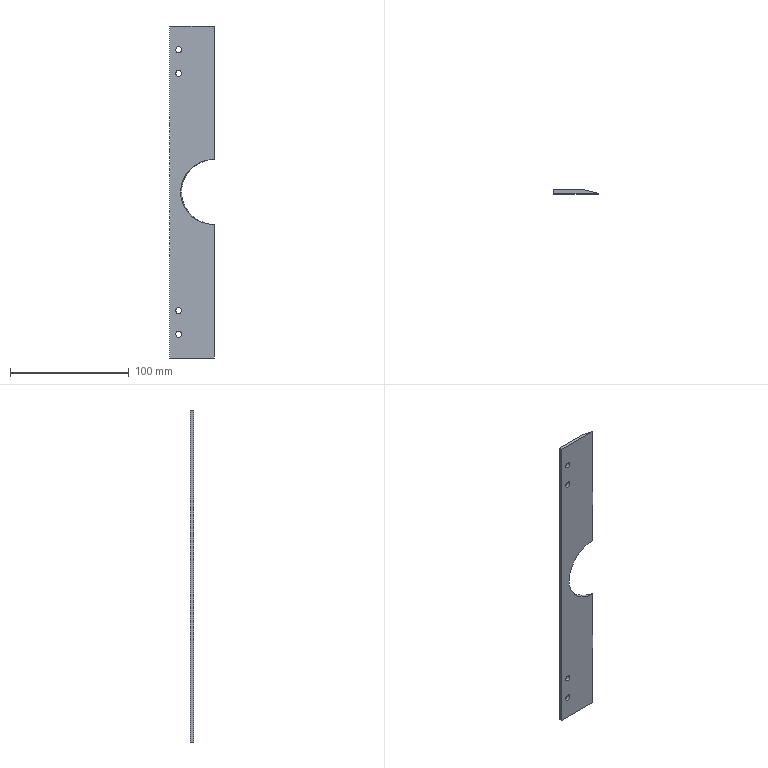Part | SolidWorks | features Cut 1, Extrusion 1, ICE 1 | 1 solid | 17 faces | box 37.5 x 3 x 280 mm | volume 23848 mm3 | cylinder 10 | plane 7 | commonest cylinder face diameters 5 x8 55 x2
STEP:
#1=CARTESIAN_POINT('',(9.03,-3.,140.));
#2=VERTEX_POINT('',#1);
#3=CARTESIAN_POINT('',(37.5,-3.,167.5));
#4=VERTEX_POINT('',#3);
#5=CARTESIAN_POINT('',(9.03,-3.,140.));
#6=CARTESIAN_POINT('',(9.03,-3.,156.109));
#7=CARTESIAN_POINT('',(20.823,-3.,167.5));
#8=CARTESIAN_POINT('',(37.5,-3.,167.5));
#9=(BOUNDED_CURVE()B_SPLINE_CURVE(3,(#5,#6,#7,#8),.UNSPECIFIED.,.F.,.F.)B_SPLINE_CURVE_WITH_KNOTS((4,4),(3.142,4.712),.UNSPECIFIED.)CURVE()GEOMETRIC_REPRESENTATION_ITEM()RATIONAL_B_SPLINE_CURVE((1.,0.8047,0.8047,1.))REPRESENTATION_ITEM(''));
#10=EDGE_CURVE('',#2,#4,#9,.T.);
#11=ORIENTED_EDGE('',*,*,#10,.F.);
#12=CARTESIAN_POINT('',(9.834,0.,140.));
#13=VERTEX_POINT('',#12);
#14=CARTESIAN_POINT('',(8.425,-5.257,140.));
#15=DIRECTION('',(0.2588,0.9659,0.));
#16=VECTOR('',#15,1000.);
#17=LINE('',#14,#16);
#18=EDGE_CURVE('',#2,#13,#17,.T.);
#19=ORIENTED_EDGE('',*,*,#18,.T.);
#20=CARTESIAN_POINT('',(26.304,0.,164.938));
#21=VERTEX_POINT('',#20);
#22=CARTESIAN_POINT('',(26.304,0.,164.938));
#23=CARTESIAN_POINT('',(15.965,0.,160.296));
#24=CARTESIAN_POINT('',(9.834,0.,151.012));
#25=CARTESIAN_POINT('',(9.834,0.,140.));
#26=(BOUNDED_CURVE()B_SPLINE_CURVE(3,(#22,#23,#24,#25),.UNSPECIFIED.,.F.,.F.)B_SPLINE_CURVE_WITH_KNOTS((4,4),(2.006,3.142),.UNSPECIFIED.)CURVE()GEOMETRIC_REPRESENTATION_ITEM()RATIONAL_B_SPLINE_CURVE((1.,0.8954,0.8954,1.))REPRESENTATION_ITEM(''));
#27=EDGE_CURVE('',#21,#13,#26,.T.);
#28=ORIENTED_EDGE('',*,*,#27,.F.);
#29=CARTESIAN_POINT('',(37.5,-3.,140.));
#30=DIRECTION('',(0.2588,0.9659,0.));
#31=DIRECTION('',(-0.9659,0.2588,0.));
#32=AXIS2_PLACEMENT_3D('',#29,#30,#31);
#33=CIRCLE('',#32,27.5);
#34=EDGE_CURVE('',#21,#4,#33,.T.);
#35=ORIENTED_EDGE('',*,*,#34,.T.);
#36=EDGE_LOOP('',(#11,#19,#28,#35));
#37=FACE_OUTER_BOUND('',#36,.T.);
#38=CARTESIAN_POINT('',(34.988,-12.375,140.));
#39=DIRECTION('',(0.2588,0.9659,0.));
#40=DIRECTION('',(-0.9659,0.2588,0.));
#41=AXIS2_PLACEMENT_3D('',#38,#39,#40);
#42=CYLINDRICAL_SURFACE('',#41,27.5);
#43=ADVANCED_FACE('',(#37),#42,.F.);
#44=CARTESIAN_POINT('',(10.,-3.,260.));
#45=VERTEX_POINT('',#44);
#46=CARTESIAN_POINT('',(5.,-3.,260.));
#47=VERTEX_POINT('',#46);
#48=CARTESIAN_POINT('',(7.5,-3.,260.));
#49=DIRECTION('',(0.,1.,0.));
#50=DIRECTION('',(0.,0.,1.));
#51=AXIS2_PLACEMENT_3D('',#48,#49,#50);
#52=CIRCLE('',#51,2.5);
#53=EDGE_CURVE('',#45,#47,#52,.T.);
#54=ORIENTED_EDGE('',*,*,#53,.F.);
#55=CARTESIAN_POINT('',(10.,0.,260.));
#56=VERTEX_POINT('',#55);
#57=CARTESIAN_POINT('',(10.,-280.,260.));
#58=DIRECTION('',(0.,1.,0.));
#59=VECTOR('',#58,1000.);
#60=LINE('',#57,#59);
#61=EDGE_CURVE('',#45,#56,#60,.T.);
#62=ORIENTED_EDGE('',*,*,#61,.T.);
#63=CARTESIAN_POINT('',(5.,0.,260.));
#64=VERTEX_POINT('',#63);
#65=CARTESIAN_POINT('',(7.5,0.,260.));
#66=DIRECTION('',(0.,1.,0.));
#67=DIRECTION('',(-1.,0.,0.));
#68=AXIS2_PLACEMENT_3D('',#65,#66,#67);
#69=CIRCLE('',#68,2.5);
#70=EDGE_CURVE('',#56,#64,#69,.T.);
#71=ORIENTED_EDGE('',*,*,#70,.T.);
#72=CARTESIAN_POINT('',(5.,-280.,260.));
#73=DIRECTION('',(0.,1.,0.));
#74=VECTOR('',#73,1000.);
#75=LINE('',#72,#74);
#76=EDGE_CURVE('',#47,#64,#75,.T.);
#77=ORIENTED_EDGE('',*,*,#76,.F.);
#78=EDGE_LOOP('',(#54,#62,#71,#77));
#79=FACE_OUTER_BOUND('',#78,.T.);
#80=CARTESIAN_POINT('',(7.5,-280.,260.));
#81=DIRECTION('',(0.,1.,0.));
#82=DIRECTION('',(-1.,0.,0.));
#83=AXIS2_PLACEMENT_3D('',#80,#81,#82);
#84=CYLINDRICAL_SURFACE('',#83,2.5);
#85=ADVANCED_FACE('',(#79),#84,.F.);
#86=CARTESIAN_POINT('',(10.,-3.,40.));
#87=VERTEX_POINT('',#86);
#88=CARTESIAN_POINT('',(5.,-3.,40.));
#89=VERTEX_POINT('',#88);
#90=CARTESIAN_POINT('',(7.5,-3.,40.));
#91=DIRECTION('',(0.,1.,0.));
#92=DIRECTION('',(0.,0.,1.));
#93=AXIS2_PLACEMENT_3D('',#90,#91,#92);
#94=CIRCLE('',#93,2.5);
#95=EDGE_CURVE('',#87,#89,#94,.T.);
#96=ORIENTED_EDGE('',*,*,#95,.F.);
#97=CARTESIAN_POINT('',(10.,0.,40.));
#98=VERTEX_POINT('',#97);
#99=CARTESIAN_POINT('',(10.,-280.,40.));
#100=DIRECTION('',(0.,1.,0.));
#101=VECTOR('',#100,1000.);
#102=LINE('',#99,#101);
#103=EDGE_CURVE('',#87,#98,#102,.T.);
#104=ORIENTED_EDGE('',*,*,#103,.T.);
#105=CARTESIAN_POINT('',(5.,0.,40.));
#106=VERTEX_POINT('',#105);
#107=CARTESIAN_POINT('',(7.5,0.,40.));
#108=DIRECTION('',(0.,1.,0.));
#109=DIRECTION('',(-1.,0.,0.));
#110=AXIS2_PLACEMENT_3D('',#107,#108,#109);
#111=CIRCLE('',#110,2.5);
#112=EDGE_CURVE('',#98,#106,#111,.T.);
#113=ORIENTED_EDGE('',*,*,#112,.T.);
#114=CARTESIAN_POINT('',(5.,-280.,40.));
#115=DIRECTION('',(0.,1.,0.));
#116=VECTOR('',#115,1000.);
#117=LINE('',#114,#116);
#118=EDGE_CURVE('',#89,#106,#117,.T.);
#119=ORIENTED_EDGE('',*,*,#118,.F.);
#120=EDGE_LOOP('',(#96,#104,#113,#119));
#121=FACE_OUTER_BOUND('',#120,.T.);
#122=CARTESIAN_POINT('',(7.5,-280.,40.));
#123=DIRECTION('',(0.,1.,0.));
#124=DIRECTION('',(-1.,0.,0.));
#125=AXIS2_PLACEMENT_3D('',#122,#123,#124);
#126=CYLINDRICAL_SURFACE('',#125,2.5);
#127=ADVANCED_FACE('',(#121),#126,.F.);
#128=CARTESIAN_POINT('',(10.,-3.,20.));
#129=VERTEX_POINT('',#128);
#130=CARTESIAN_POINT('',(5.,-3.,20.));
#131=VERTEX_POINT('',#130);
#132=CARTESIAN_POINT('',(7.5,-3.,20.));
#133=DIRECTION('',(0.,1.,0.));
#134=DIRECTION('',(0.,0.,1.));
#135=AXIS2_PLACEMENT_3D('',#132,#133,#134);
#136=CIRCLE('',#135,2.5);
#137=EDGE_CURVE('',#129,#131,#136,.T.);
#138=ORIENTED_EDGE('',*,*,#137,.F.);
#139=CARTESIAN_POINT('',(10.,0.,20.));
#140=VERTEX_POINT('',#139);
#141=CARTESIAN_POINT('',(10.,-280.,20.));
#142=DIRECTION('',(0.,1.,0.));
#143=VECTOR('',#142,1000.);
#144=LINE('',#141,#143);
#145=EDGE_CURVE('',#129,#140,#144,.T.);
#146=ORIENTED_EDGE('',*,*,#145,.T.);
#147=CARTESIAN_POINT('',(5.,0.,20.));
#148=VERTEX_POINT('',#147);
#149=CARTESIAN_POINT('',(7.5,0.,20.));
#150=DIRECTION('',(0.,1.,0.));
#151=DIRECTION('',(-1.,0.,0.));
#152=AXIS2_PLACEMENT_3D('',#149,#150,#151);
#153=CIRCLE('',#152,2.5);
#154=EDGE_CURVE('',#140,#148,#153,.T.);
#155=ORIENTED_EDGE('',*,*,#154,.T.);
#156=CARTESIAN_POINT('',(5.,-280.,20.));
#157=DIRECTION('',(0.,1.,0.));
#158=VECTOR('',#157,1000.);
#159=LINE('',#156,#158);
#160=EDGE_CURVE('',#131,#148,#159,.T.);
#161=ORIENTED_EDGE('',*,*,#160,.F.);
#162=EDGE_LOOP('',(#138,#146,#155,#161));
#163=FACE_OUTER_BOUND('',#162,.T.);
#164=CARTESIAN_POINT('',(7.5,-280.,20.));
#165=DIRECTION('',(0.,1.,0.));
#166=DIRECTION('',(-1.,0.,0.));
#167=AXIS2_PLACEMENT_3D('',#164,#165,#166);
#168=CYLINDRICAL_SURFACE('',#167,2.5);
#169=ADVANCED_FACE('',(#163),#168,.F.);
#170=CARTESIAN_POINT('',(10.,-3.,240.));
#171=VERTEX_POINT('',#170);
#172=CARTESIAN_POINT('',(5.,-3.,240.));
#173=VERTEX_POINT('',#172);
#174=CARTESIAN_POINT('',(7.5,-3.,240.));
#175=DIRECTION('',(0.,1.,0.));
#176=DIRECTION('',(0.,0.,1.));
#177=AXIS2_PLACEMENT_3D('',#174,#175,#176);
#178=CIRCLE('',#177,2.5);
#179=EDGE_CURVE('',#171,#173,#178,.T.);
#180=ORIENTED_EDGE('',*,*,#179,.F.);
#181=CARTESIAN_POINT('',(10.,0.,240.));
#182=VERTEX_POINT('',#181);
#183=CARTESIAN_POINT('',(10.,-280.,240.));
#184=DIRECTION('',(0.,1.,0.));
#185=VECTOR('',#184,1000.);
#186=LINE('',#183,#185);
#187=EDGE_CURVE('',#171,#182,#186,.T.);
#188=ORIENTED_EDGE('',*,*,#187,.T.);
#189=CARTESIAN_POINT('',(5.,0.,240.));
#190=VERTEX_POINT('',#189);
#191=CARTESIAN_POINT('',(7.5,0.,240.));
#192=DIRECTION('',(0.,1.,0.));
#193=DIRECTION('',(-1.,0.,0.));
#194=AXIS2_PLACEMENT_3D('',#191,#192,#193);
#195=CIRCLE('',#194,2.5);
#196=EDGE_CURVE('',#182,#190,#195,.T.);
#197=ORIENTED_EDGE('',*,*,#196,.T.);
#198=CARTESIAN_POINT('',(5.,-280.,240.));
#199=DIRECTION('',(0.,1.,0.));
#200=VECTOR('',#199,1000.);
#201=LINE('',#198,#200);
#202=EDGE_CURVE('',#173,#190,#201,.T.);
#203=ORIENTED_EDGE('',*,*,#202,.F.);
#204=EDGE_LOOP('',(#180,#188,#197,#203));
#205=FACE_OUTER_BOUND('',#204,.T.);
#206=CARTESIAN_POINT('',(7.5,-280.,240.));
#207=DIRECTION('',(0.,1.,0.));
#208=DIRECTION('',(-1.,0.,0.));
#209=AXIS2_PLACEMENT_3D('',#206,#207,#208);
#210=CYLINDRICAL_SURFACE('',#209,2.5);
#211=ADVANCED_FACE('',(#205),#210,.F.);
#212=CARTESIAN_POINT('',(37.5,-3.,280.));
#213=VERTEX_POINT('',#212);
#214=CARTESIAN_POINT('',(37.5,-3.,280.));
#215=DIRECTION('',(0.,0.,-1.));
#216=VECTOR('',#215,1000.);
#217=LINE('',#214,#216);
#218=EDGE_CURVE('',#213,#4,#217,.T.);
#219=ORIENTED_EDGE('',*,*,#218,.T.);
#220=ORIENTED_EDGE('',*,*,#34,.F.);
#221=CARTESIAN_POINT('',(26.304,0.,280.));
#222=VERTEX_POINT('',#221);
#223=CARTESIAN_POINT('',(26.304,0.,280.));
#224=DIRECTION('',(0.,0.,-1.));
#225=VECTOR('',#224,1000.);
#226=LINE('',#223,#225);
#227=EDGE_CURVE('',#222,#21,#226,.T.);
#228=ORIENTED_EDGE('',*,*,#227,.F.);
#229=CARTESIAN_POINT('',(37.5,-3.,280.));
#230=DIRECTION('',(-0.9659,0.2588,0.));
#231=VECTOR('',#230,1000.);
#232=LINE('',#229,#231);
#233=EDGE_CURVE('',#213,#222,#232,.T.);
#234=ORIENTED_EDGE('',*,*,#233,.F.);
#235=EDGE_LOOP('',(#219,#220,#228,#234));
#236=FACE_OUTER_BOUND('',#235,.T.);
#237=CARTESIAN_POINT('',(37.5,-3.,280.));
#238=DIRECTION('',(-0.2588,-0.9659,0.));
#239=DIRECTION('',(0.9659,-0.2588,0.));
#240=AXIS2_PLACEMENT_3D('',#237,#238,#239);
#241=PLANE('',#240);
#242=ADVANCED_FACE('',(#236),#241,.F.);
#243=CARTESIAN_POINT('',(7.5,0.,260.));
#244=DIRECTION('',(0.,1.,0.));
#245=DIRECTION('',(-1.,0.,0.));
#246=AXIS2_PLACEMENT_3D('',#243,#244,#245);
#247=CIRCLE('',#246,2.5);
#248=EDGE_CURVE('',#64,#56,#247,.T.);
#249=ORIENTED_EDGE('',*,*,#248,.F.);
#250=ORIENTED_EDGE('',*,*,#70,.F.);
#251=EDGE_LOOP('',(#249,#250));
#252=FACE_BOUND('',#251,.T.);
#253=CARTESIAN_POINT('',(7.5,0.,40.));
#254=DIRECTION('',(0.,1.,0.));
#255=DIRECTION('',(-1.,0.,0.));
#256=AXIS2_PLACEMENT_3D('',#253,#254,#255);
#257=CIRCLE('',#256,2.5);
#258=EDGE_CURVE('',#106,#98,#257,.T.);
#259=ORIENTED_EDGE('',*,*,#258,.F.);
#260=ORIENTED_EDGE('',*,*,#112,.F.);
#261=EDGE_LOOP('',(#259,#260));
#262=FACE_BOUND('',#261,.T.);
#263=CARTESIAN_POINT('',(7.5,0.,20.));
#264=DIRECTION('',(0.,1.,0.));
#265=DIRECTION('',(-1.,0.,0.));
#266=AXIS2_PLACEMENT_3D('',#263,#264,#265);
#267=CIRCLE('',#266,2.5);
#268=EDGE_CURVE('',#148,#140,#267,.T.);
#269=ORIENTED_EDGE('',*,*,#268,.F.);
#270=ORIENTED_EDGE('',*,*,#154,.F.);
#271=EDGE_LOOP('',(#269,#270));
#272=FACE_BOUND('',#271,.T.);
#273=CARTESIAN_POINT('',(7.5,0.,240.));
#274=DIRECTION('',(0.,1.,0.));
#275=DIRECTION('',(-1.,0.,0.));
#276=AXIS2_PLACEMENT_3D('',#273,#274,#275);
#277=CIRCLE('',#276,2.5);
#278=EDGE_CURVE('',#190,#182,#277,.T.);
#279=ORIENTED_EDGE('',*,*,#278,.F.);
#280=ORIENTED_EDGE('',*,*,#196,.F.);
#281=EDGE_LOOP('',(#279,#280));
#282=FACE_BOUND('',#281,.T.);
#283=ORIENTED_EDGE('',*,*,#227,.T.);
#284=ORIENTED_EDGE('',*,*,#27,.T.);
#285=CARTESIAN_POINT('',(26.304,0.,115.062));
#286=VERTEX_POINT('',#285);
#287=CARTESIAN_POINT('',(9.834,0.,140.));
#288=CARTESIAN_POINT('',(9.834,0.,128.988));
#289=CARTESIAN_POINT('',(15.965,0.,119.704));
#290=CARTESIAN_POINT('',(26.304,0.,115.062));
#291=(BOUNDED_CURVE()B_SPLINE_CURVE(3,(#287,#288,#289,#290),.UNSPECIFIED.,.F.,.F.)B_SPLINE_CURVE_WITH_KNOTS((4,4),(3.142,4.277),.UNSPECIFIED.)CURVE()GEOMETRIC_REPRESENTATION_ITEM()RATIONAL_B_SPLINE_CURVE((1.,0.8954,0.8954,1.))REPRESENTATION_ITEM(''));
#292=EDGE_CURVE('',#13,#286,#291,.T.);
#293=ORIENTED_EDGE('',*,*,#292,.T.);
#294=CARTESIAN_POINT('',(26.304,0.,0.));
#295=VERTEX_POINT('',#294);
#296=CARTESIAN_POINT('',(26.304,0.,280.));
#297=DIRECTION('',(0.,0.,-1.));
#298=VECTOR('',#297,1000.);
#299=LINE('',#296,#298);
#300=EDGE_CURVE('',#286,#295,#299,.T.);
#301=ORIENTED_EDGE('',*,*,#300,.T.);
#302=CARTESIAN_POINT('',(0.,0.,0.));
#303=VERTEX_POINT('',#302);
#304=CARTESIAN_POINT('',(26.304,0.,0.));
#305=DIRECTION('',(-1.,0.,0.));
#306=VECTOR('',#305,1000.);
#307=LINE('',#304,#306);
#308=EDGE_CURVE('',#295,#303,#307,.T.);
#309=ORIENTED_EDGE('',*,*,#308,.T.);
#310=CARTESIAN_POINT('',(0.,0.,280.));
#311=VERTEX_POINT('',#310);
#312=CARTESIAN_POINT('',(0.,0.,280.));
#313=DIRECTION('',(0.,0.,-1.));
#314=VECTOR('',#313,1000.);
#315=LINE('',#312,#314);
#316=EDGE_CURVE('',#311,#303,#315,.T.);
#317=ORIENTED_EDGE('',*,*,#316,.F.);
#318=CARTESIAN_POINT('',(26.304,0.,280.));
#319=DIRECTION('',(-1.,0.,0.));
#320=VECTOR('',#319,1000.);
#321=LINE('',#318,#320);
#322=EDGE_CURVE('',#222,#311,#321,.T.);
#323=ORIENTED_EDGE('',*,*,#322,.F.);
#324=EDGE_LOOP('',(#283,#284,#293,#301,#309,#317,#323));
#325=FACE_OUTER_BOUND('',#324,.T.);
#326=CARTESIAN_POINT('',(26.304,0.,280.));
#327=DIRECTION('',(0.,-1.,0.));
#328=DIRECTION('',(1.,0.,0.));
#329=AXIS2_PLACEMENT_3D('',#326,#327,#328);
#330=PLANE('',#329);
#331=ADVANCED_FACE('',(#252,#262,#272,#282,#325),#330,.F.);
#332=CARTESIAN_POINT('',(0.,-3.,0.));
#333=VERTEX_POINT('',#332);
#334=CARTESIAN_POINT('',(0.,0.,0.));
#335=DIRECTION('',(0.,-1.,0.));
#336=VECTOR('',#335,1000.);
#337=LINE('',#334,#336);
#338=EDGE_CURVE('',#303,#333,#337,.T.);
#339=ORIENTED_EDGE('',*,*,#338,.T.);
#340=CARTESIAN_POINT('',(0.,-3.,280.));
#341=VERTEX_POINT('',#340);
#342=CARTESIAN_POINT('',(0.,-3.,280.));
#343=DIRECTION('',(0.,0.,-1.));
#344=VECTOR('',#343,1000.);
#345=LINE('',#342,#344);
#346=EDGE_CURVE('',#341,#333,#345,.T.);
#347=ORIENTED_EDGE('',*,*,#346,.F.);
#348=CARTESIAN_POINT('',(0.,0.,280.));
#349=DIRECTION('',(0.,-1.,0.));
#350=VECTOR('',#349,1000.);
#351=LINE('',#348,#350);
#352=EDGE_CURVE('',#311,#341,#351,.T.);
#353=ORIENTED_EDGE('',*,*,#352,.F.);
#354=ORIENTED_EDGE('',*,*,#316,.T.);
#355=EDGE_LOOP('',(#339,#347,#353,#354));
#356=FACE_OUTER_BOUND('',#355,.T.);
#357=CARTESIAN_POINT('',(0.,0.,280.));
#358=DIRECTION('',(1.,0.,0.));
#359=DIRECTION('',(0.,1.,0.));
#360=AXIS2_PLACEMENT_3D('',#357,#358,#359);
#361=PLANE('',#360);
#362=ADVANCED_FACE('',(#356),#361,.F.);
#363=CARTESIAN_POINT('',(7.5,-3.,260.));
#364=DIRECTION('',(0.,1.,0.));
#365=DIRECTION('',(0.,0.,1.));
#366=AXIS2_PLACEMENT_3D('',#363,#364,#365);
#367=CIRCLE('',#366,2.5);
#368=EDGE_CURVE('',#47,#45,#367,.T.);
#369=ORIENTED_EDGE('',*,*,#368,.T.);
#370=ORIENTED_EDGE('',*,*,#53,.T.);
#371=EDGE_LOOP('',(#369,#370));
#372=FACE_BOUND('',#371,.T.);
#373=CARTESIAN_POINT('',(7.5,-3.,40.));
#374=DIRECTION('',(0.,1.,0.));
#375=DIRECTION('',(0.,0.,1.));
#376=AXIS2_PLACEMENT_3D('',#373,#374,#375);
#377=CIRCLE('',#376,2.5);
#378=EDGE_CURVE('',#89,#87,#377,.T.);
#379=ORIENTED_EDGE('',*,*,#378,.T.);
#380=ORIENTED_EDGE('',*,*,#95,.T.);
#381=EDGE_LOOP('',(#379,#380));
#382=FACE_BOUND('',#381,.T.);
#383=CARTESIAN_POINT('',(7.5,-3.,20.));
#384=DIRECTION('',(0.,1.,0.));
#385=DIRECTION('',(0.,0.,1.));
#386=AXIS2_PLACEMENT_3D('',#383,#384,#385);
#387=CIRCLE('',#386,2.5);
#388=EDGE_CURVE('',#131,#129,#387,.T.);
#389=ORIENTED_EDGE('',*,*,#388,.T.);
#390=ORIENTED_EDGE('',*,*,#137,.T.);
#391=EDGE_LOOP('',(#389,#390));
#392=FACE_BOUND('',#391,.T.);
#393=CARTESIAN_POINT('',(7.5,-3.,240.));
#394=DIRECTION('',(0.,1.,0.));
#395=DIRECTION('',(0.,0.,1.));
#396=AXIS2_PLACEMENT_3D('',#393,#394,#395);
#397=CIRCLE('',#396,2.5);
#398=EDGE_CURVE('',#173,#171,#397,.T.);
#399=ORIENTED_EDGE('',*,*,#398,.T.);
#400=ORIENTED_EDGE('',*,*,#179,.T.);
#401=EDGE_LOOP('',(#399,#400));
#402=FACE_BOUND('',#401,.T.);
#403=CARTESIAN_POINT('',(37.5,-3.,112.5));
#404=VERTEX_POINT('',#403);
#405=CARTESIAN_POINT('',(37.5,-3.,0.));
#406=VERTEX_POINT('',#405);
#407=CARTESIAN_POINT('',(37.5,-3.,280.));
#408=DIRECTION('',(0.,0.,-1.));
#409=VECTOR('',#408,1000.);
#410=LINE('',#407,#409);
#411=EDGE_CURVE('',#404,#406,#410,.T.);
#412=ORIENTED_EDGE('',*,*,#411,.F.);
#413=CARTESIAN_POINT('',(37.5,-3.,112.5));
#414=CARTESIAN_POINT('',(20.823,-3.,112.5));
#415=CARTESIAN_POINT('',(9.03,-3.,123.891));
#416=CARTESIAN_POINT('',(9.03,-3.,140.));
#417=(BOUNDED_CURVE()B_SPLINE_CURVE(3,(#413,#414,#415,#416),.UNSPECIFIED.,.F.,.F.)B_SPLINE_CURVE_WITH_KNOTS((4,4),(1.571,3.142),.UNSPECIFIED.)CURVE()GEOMETRIC_REPRESENTATION_ITEM()RATIONAL_B_SPLINE_CURVE((1.,0.8047,0.8047,1.))REPRESENTATION_ITEM(''));
#418=EDGE_CURVE('',#404,#2,#417,.T.);
#419=ORIENTED_EDGE('',*,*,#418,.T.);
#420=ORIENTED_EDGE('',*,*,#10,.T.);
#421=ORIENTED_EDGE('',*,*,#218,.F.);
#422=CARTESIAN_POINT('',(0.,-3.,280.));
#423=DIRECTION('',(1.,0.,0.));
#424=VECTOR('',#423,1000.);
#425=LINE('',#422,#424);
#426=EDGE_CURVE('',#341,#213,#425,.T.);
#427=ORIENTED_EDGE('',*,*,#426,.F.);
#428=ORIENTED_EDGE('',*,*,#346,.T.);
#429=CARTESIAN_POINT('',(0.,-3.,0.));
#430=DIRECTION('',(1.,0.,0.));
#431=VECTOR('',#430,1000.);
#432=LINE('',#429,#431);
#433=EDGE_CURVE('',#333,#406,#432,.T.);
#434=ORIENTED_EDGE('',*,*,#433,.T.);
#435=EDGE_LOOP('',(#412,#419,#420,#421,#427,#428,#434));
#436=FACE_OUTER_BOUND('',#435,.T.);
#437=CARTESIAN_POINT('',(0.,-3.,280.));
#438=DIRECTION('',(0.,1.,0.));
#439=DIRECTION('',(0.,0.,1.));
#440=AXIS2_PLACEMENT_3D('',#437,#438,#439);
#441=PLANE('',#440);
#442=ADVANCED_FACE('',(#372,#382,#392,#402,#436),#441,.F.);
#443=ORIENTED_EDGE('',*,*,#300,.F.);
#444=CARTESIAN_POINT('',(37.5,-3.,140.));
#445=DIRECTION('',(-0.2588,-0.9659,0.));
#446=DIRECTION('',(0.9659,-0.2588,0.));
#447=AXIS2_PLACEMENT_3D('',#444,#445,#446);
#448=CIRCLE('',#447,27.5);
#449=EDGE_CURVE('',#286,#404,#448,.T.);
#450=ORIENTED_EDGE('',*,*,#449,.T.);
#451=ORIENTED_EDGE('',*,*,#411,.T.);
#452=CARTESIAN_POINT('',(37.5,-3.,0.));
#453=DIRECTION('',(-0.9659,0.2588,0.));
#454=VECTOR('',#453,1000.);
#455=LINE('',#452,#454);
#456=EDGE_CURVE('',#406,#295,#455,.T.);
#457=ORIENTED_EDGE('',*,*,#456,.T.);
#458=EDGE_LOOP('',(#443,#450,#451,#457));
#459=FACE_OUTER_BOUND('',#458,.T.);
#460=CARTESIAN_POINT('',(37.5,-3.,280.));
#461=DIRECTION('',(-0.2588,-0.9659,0.));
#462=DIRECTION('',(0.9659,-0.2588,0.));
#463=AXIS2_PLACEMENT_3D('',#460,#461,#462);
#464=PLANE('',#463);
#465=ADVANCED_FACE('',(#459),#464,.F.);
#466=ORIENTED_EDGE('',*,*,#322,.T.);
#467=ORIENTED_EDGE('',*,*,#352,.T.);
#468=ORIENTED_EDGE('',*,*,#426,.T.);
#469=ORIENTED_EDGE('',*,*,#233,.T.);
#470=EDGE_LOOP('',(#466,#467,#468,#469));
#471=FACE_OUTER_BOUND('',#470,.T.);
#472=CARTESIAN_POINT('',(0.,0.,280.));
#473=DIRECTION('',(0.,0.,1.));
#474=DIRECTION('',(1.,0.,0.));
#475=AXIS2_PLACEMENT_3D('',#472,#473,#474);
#476=PLANE('',#475);
#477=ADVANCED_FACE('',(#471),#476,.T.);
#478=ORIENTED_EDGE('',*,*,#308,.F.);
#479=ORIENTED_EDGE('',*,*,#456,.F.);
#480=ORIENTED_EDGE('',*,*,#433,.F.);
#481=ORIENTED_EDGE('',*,*,#338,.F.);
#482=EDGE_LOOP('',(#478,#479,#480,#481));
#483=FACE_OUTER_BOUND('',#482,.T.);
#484=CARTESIAN_POINT('',(0.,0.,0.));
#485=DIRECTION('',(0.,0.,1.));
#486=DIRECTION('',(1.,0.,0.));
#487=AXIS2_PLACEMENT_3D('',#484,#485,#486);
#488=PLANE('',#487);
#489=ADVANCED_FACE('',(#483),#488,.F.);
#490=ORIENTED_EDGE('',*,*,#187,.F.);
#491=ORIENTED_EDGE('',*,*,#398,.F.);
#492=ORIENTED_EDGE('',*,*,#202,.T.);
#493=ORIENTED_EDGE('',*,*,#278,.T.);
#494=EDGE_LOOP('',(#490,#491,#492,#493));
#495=FACE_OUTER_BOUND('',#494,.T.);
#496=CARTESIAN_POINT('',(7.5,-280.,240.));
#497=DIRECTION('',(0.,1.,0.));
#498=DIRECTION('',(-1.,0.,0.));
#499=AXIS2_PLACEMENT_3D('',#496,#497,#498);
#500=CYLINDRICAL_SURFACE('',#499,2.5);
#501=ADVANCED_FACE('',(#495),#500,.F.);
#502=ORIENTED_EDGE('',*,*,#145,.F.);
#503=ORIENTED_EDGE('',*,*,#388,.F.);
#504=ORIENTED_EDGE('',*,*,#160,.T.);
#505=ORIENTED_EDGE('',*,*,#268,.T.);
#506=EDGE_LOOP('',(#502,#503,#504,#505));
#507=FACE_OUTER_BOUND('',#506,.T.);
#508=CARTESIAN_POINT('',(7.5,-280.,20.));
#509=DIRECTION('',(0.,1.,0.));
#510=DIRECTION('',(-1.,0.,0.));
#511=AXIS2_PLACEMENT_3D('',#508,#509,#510);
#512=CYLINDRICAL_SURFACE('',#511,2.5);
#513=ADVANCED_FACE('',(#507),#512,.F.);
#514=ORIENTED_EDGE('',*,*,#103,.F.);
#515=ORIENTED_EDGE('',*,*,#378,.F.);
#516=ORIENTED_EDGE('',*,*,#118,.T.);
#517=ORIENTED_EDGE('',*,*,#258,.T.);
#518=EDGE_LOOP('',(#514,#515,#516,#517));
#519=FACE_OUTER_BOUND('',#518,.T.);
#520=CARTESIAN_POINT('',(7.5,-280.,40.));
#521=DIRECTION('',(0.,1.,0.));
#522=DIRECTION('',(-1.,0.,0.));
#523=AXIS2_PLACEMENT_3D('',#520,#521,#522);
#524=CYLINDRICAL_SURFACE('',#523,2.5);
#525=ADVANCED_FACE('',(#519),#524,.F.);
#526=ORIENTED_EDGE('',*,*,#61,.F.);
#527=ORIENTED_EDGE('',*,*,#368,.F.);
#528=ORIENTED_EDGE('',*,*,#76,.T.);
#529=ORIENTED_EDGE('',*,*,#248,.T.);
#530=EDGE_LOOP('',(#526,#527,#528,#529));
#531=FACE_OUTER_BOUND('',#530,.T.);
#532=CARTESIAN_POINT('',(7.5,-280.,260.));
#533=DIRECTION('',(0.,1.,0.));
#534=DIRECTION('',(-1.,0.,0.));
#535=AXIS2_PLACEMENT_3D('',#532,#533,#534);
#536=CYLINDRICAL_SURFACE('',#535,2.5);
#537=ADVANCED_FACE('',(#531),#536,.F.);
#538=ORIENTED_EDGE('',*,*,#18,.F.);
#539=ORIENTED_EDGE('',*,*,#418,.F.);
#540=ORIENTED_EDGE('',*,*,#449,.F.);
#541=ORIENTED_EDGE('',*,*,#292,.F.);
#542=EDGE_LOOP('',(#538,#539,#540,#541));
#543=FACE_OUTER_BOUND('',#542,.T.);
#544=CARTESIAN_POINT('',(34.988,-12.375,140.));
#545=DIRECTION('',(0.2588,0.9659,0.));
#546=DIRECTION('',(-0.9659,0.2588,0.));
#547=AXIS2_PLACEMENT_3D('',#544,#545,#546);
#548=CYLINDRICAL_SURFACE('',#547,27.5);
#549=ADVANCED_FACE('',(#543),#548,.F.);
#550=CLOSED_SHELL('',(#43,#85,#127,#169,#211,#242,#331,#362,#442,#465,#477,#489,#501,#513,#525,#537,#549));
#551=MANIFOLD_SOLID_BREP('',#550);
#552=CARTESIAN_POINT('',(0.,0.,0.));
#553=DIRECTION('',(0.,0.,1.));
#554=DIRECTION('',(1.,0.,0.));
#555=AXIS2_PLACEMENT_3D('',#552,#553,#554);
#556=(LENGTH_UNIT()NAMED_UNIT(*)SI_UNIT(.MILLI.,.METRE.));
#557=UNCERTAINTY_MEASURE_WITH_UNIT(LENGTH_MEASURE(0.00001),#556,'','');
#558=(NAMED_UNIT(*)PLANE_ANGLE_UNIT()SI_UNIT($,.RADIAN.));
#559=(NAMED_UNIT(*)SI_UNIT($,.STERADIAN.)SOLID_ANGLE_UNIT());
#560=(GEOMETRIC_REPRESENTATION_CONTEXT(3)GLOBAL_UNCERTAINTY_ASSIGNED_CONTEXT((#557))GLOBAL_UNIT_ASSIGNED_CONTEXT((#556,#558,#559))REPRESENTATION_CONTEXT('',''));
#561=ADVANCED_BREP_SHAPE_REPRESENTATION('',(#551,#555),#560);